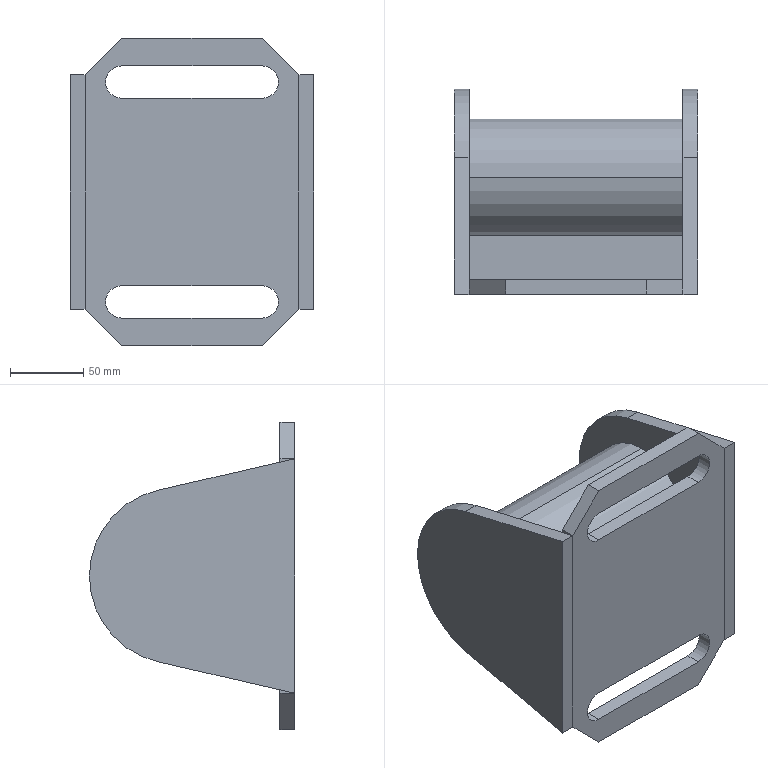Part | SolidWorks | features MirrorStock 1 | 5 solids | 42 faces | box 166 x 140 x 210 mm | volume 892301 mm3 | plane 31 | cylinder 11 | commonest cylinder face diameters 22 x4 80 x3 64 x2 120 x2
STEP:
#1=CARTESIAN_POINT('',(-48.,10.,105.));
#2=VERTEX_POINT('',#1);
#3=CARTESIAN_POINT('',(-73.,10.,80.));
#4=VERTEX_POINT('',#3);
#5=CARTESIAN_POINT('',(-73.,10.,80.));
#6=DIRECTION('',(-0.7071,0.,-0.7071));
#7=VECTOR('',#6,1000.);
#8=LINE('',#5,#7);
#9=EDGE_CURVE('',#2,#4,#8,.T.);
#10=ORIENTED_EDGE('',*,*,#9,.F.);
#11=CARTESIAN_POINT('',(48.,10.,105.));
#12=VERTEX_POINT('',#11);
#13=CARTESIAN_POINT('',(-48.,10.,105.));
#14=DIRECTION('',(-1.,0.,0.));
#15=VECTOR('',#14,1000.);
#16=LINE('',#13,#15);
#17=EDGE_CURVE('',#12,#2,#16,.T.);
#18=ORIENTED_EDGE('',*,*,#17,.F.);
#19=CARTESIAN_POINT('',(73.,10.,80.));
#20=VERTEX_POINT('',#19);
#21=CARTESIAN_POINT('',(73.,10.,80.));
#22=DIRECTION('',(-0.7071,0.,0.7071));
#23=VECTOR('',#22,1000.);
#24=LINE('',#21,#23);
#25=EDGE_CURVE('',#20,#12,#24,.T.);
#26=ORIENTED_EDGE('',*,*,#25,.F.);
#27=CARTESIAN_POINT('',(73.,10.,-80.));
#28=VERTEX_POINT('',#27);
#29=CARTESIAN_POINT('',(73.,10.,-80.));
#30=DIRECTION('',(0.,0.,1.));
#31=VECTOR('',#30,1000.);
#32=LINE('',#29,#31);
#33=EDGE_CURVE('',#28,#20,#32,.T.);
#34=ORIENTED_EDGE('',*,*,#33,.F.);
#35=CARTESIAN_POINT('',(48.,10.,-105.));
#36=VERTEX_POINT('',#35);
#37=CARTESIAN_POINT('',(73.,10.,-80.));
#38=DIRECTION('',(0.7071,0.,0.7071));
#39=VECTOR('',#38,1000.);
#40=LINE('',#37,#39);
#41=EDGE_CURVE('',#36,#28,#40,.T.);
#42=ORIENTED_EDGE('',*,*,#41,.F.);
#43=CARTESIAN_POINT('',(-48.,10.,-105.));
#44=VERTEX_POINT('',#43);
#45=CARTESIAN_POINT('',(-48.,10.,-105.));
#46=DIRECTION('',(1.,0.,0.));
#47=VECTOR('',#46,1000.);
#48=LINE('',#45,#47);
#49=EDGE_CURVE('',#44,#36,#48,.T.);
#50=ORIENTED_EDGE('',*,*,#49,.F.);
#51=CARTESIAN_POINT('',(-73.,10.,-80.));
#52=VERTEX_POINT('',#51);
#53=CARTESIAN_POINT('',(-73.,10.,-80.));
#54=DIRECTION('',(0.7071,0.,-0.7071));
#55=VECTOR('',#54,1000.);
#56=LINE('',#53,#55);
#57=EDGE_CURVE('',#52,#44,#56,.T.);
#58=ORIENTED_EDGE('',*,*,#57,.F.);
#59=CARTESIAN_POINT('',(-73.,10.,-80.));
#60=DIRECTION('',(0.,0.,-1.));
#61=VECTOR('',#60,1000.);
#62=LINE('',#59,#61);
#63=EDGE_CURVE('',#4,#52,#62,.T.);
#64=ORIENTED_EDGE('',*,*,#63,.F.);
#65=EDGE_LOOP('',(#10,#18,#26,#34,#42,#50,#58,#64));
#66=FACE_OUTER_BOUND('',#65,.T.);
#67=CARTESIAN_POINT('',(-48.,10.,64.));
#68=VERTEX_POINT('',#67);
#69=CARTESIAN_POINT('',(48.,10.,64.));
#70=VERTEX_POINT('',#69);
#71=CARTESIAN_POINT('',(-48.,10.,64.));
#72=DIRECTION('',(1.,0.,0.));
#73=VECTOR('',#72,1000.);
#74=LINE('',#71,#73);
#75=EDGE_CURVE('',#68,#70,#74,.T.);
#76=ORIENTED_EDGE('',*,*,#75,.T.);
#77=CARTESIAN_POINT('',(48.,10.,86.));
#78=VERTEX_POINT('',#77);
#79=CARTESIAN_POINT('',(48.,10.,75.));
#80=DIRECTION('',(0.,-1.,0.));
#81=DIRECTION('',(0.,0.,-1.));
#82=AXIS2_PLACEMENT_3D('',#79,#80,#81);
#83=CIRCLE('',#82,11.);
#84=EDGE_CURVE('',#70,#78,#83,.T.);
#85=ORIENTED_EDGE('',*,*,#84,.T.);
#86=CARTESIAN_POINT('',(-48.,10.,86.));
#87=VERTEX_POINT('',#86);
#88=CARTESIAN_POINT('',(-48.,10.,86.));
#89=DIRECTION('',(-1.,0.,0.));
#90=VECTOR('',#89,1000.);
#91=LINE('',#88,#90);
#92=EDGE_CURVE('',#78,#87,#91,.T.);
#93=ORIENTED_EDGE('',*,*,#92,.T.);
#94=CARTESIAN_POINT('',(-48.,10.,75.));
#95=DIRECTION('',(0.,-1.,0.));
#96=DIRECTION('',(0.,0.,-1.));
#97=AXIS2_PLACEMENT_3D('',#94,#95,#96);
#98=CIRCLE('',#97,11.);
#99=EDGE_CURVE('',#87,#68,#98,.T.);
#100=ORIENTED_EDGE('',*,*,#99,.T.);
#101=EDGE_LOOP('',(#76,#85,#93,#100));
#102=FACE_BOUND('',#101,.T.);
#103=CARTESIAN_POINT('',(-48.,10.,-86.));
#104=VERTEX_POINT('',#103);
#105=CARTESIAN_POINT('',(48.,10.,-86.));
#106=VERTEX_POINT('',#105);
#107=CARTESIAN_POINT('',(-48.,10.,-86.));
#108=DIRECTION('',(1.,0.,0.));
#109=VECTOR('',#108,1000.);
#110=LINE('',#107,#109);
#111=EDGE_CURVE('',#104,#106,#110,.T.);
#112=ORIENTED_EDGE('',*,*,#111,.T.);
#113=CARTESIAN_POINT('',(48.,10.,-64.));
#114=VERTEX_POINT('',#113);
#115=CARTESIAN_POINT('',(48.,10.,-75.));
#116=DIRECTION('',(0.,-1.,0.));
#117=DIRECTION('',(0.,0.,1.));
#118=AXIS2_PLACEMENT_3D('',#115,#116,#117);
#119=CIRCLE('',#118,11.);
#120=EDGE_CURVE('',#106,#114,#119,.T.);
#121=ORIENTED_EDGE('',*,*,#120,.T.);
#122=CARTESIAN_POINT('',(-48.,10.,-64.));
#123=VERTEX_POINT('',#122);
#124=CARTESIAN_POINT('',(-48.,10.,-64.));
#125=DIRECTION('',(-1.,0.,0.));
#126=VECTOR('',#125,1000.);
#127=LINE('',#124,#126);
#128=EDGE_CURVE('',#114,#123,#127,.T.);
#129=ORIENTED_EDGE('',*,*,#128,.T.);
#130=CARTESIAN_POINT('',(-48.,10.,-75.));
#131=DIRECTION('',(0.,-1.,0.));
#132=DIRECTION('',(0.,0.,1.));
#133=AXIS2_PLACEMENT_3D('',#130,#131,#132);
#134=CIRCLE('',#133,11.);
#135=EDGE_CURVE('',#123,#104,#134,.T.);
#136=ORIENTED_EDGE('',*,*,#135,.T.);
#137=EDGE_LOOP('',(#112,#121,#129,#136));
#138=FACE_BOUND('',#137,.T.);
#139=CARTESIAN_POINT('',(0.,10.,0.));
#140=DIRECTION('',(0.,1.,0.));
#141=DIRECTION('',(0.,0.,-1.));
#142=AXIS2_PLACEMENT_3D('',#139,#140,#141);
#143=PLANE('',#142);
#144=ADVANCED_FACE('',(#66,#102,#138),#143,.T.);
#145=CARTESIAN_POINT('',(-48.,0.,86.));
#146=VERTEX_POINT('',#145);
#147=CARTESIAN_POINT('',(-48.,0.,64.));
#148=VERTEX_POINT('',#147);
#149=CARTESIAN_POINT('',(-48.,0.,75.));
#150=DIRECTION('',(0.,-1.,0.));
#151=DIRECTION('',(0.,0.,-1.));
#152=AXIS2_PLACEMENT_3D('',#149,#150,#151);
#153=CIRCLE('',#152,11.);
#154=EDGE_CURVE('',#146,#148,#153,.T.);
#155=ORIENTED_EDGE('',*,*,#154,.F.);
#156=CARTESIAN_POINT('',(48.,0.,86.));
#157=VERTEX_POINT('',#156);
#158=CARTESIAN_POINT('',(-48.,0.,86.));
#159=DIRECTION('',(-1.,0.,0.));
#160=VECTOR('',#159,1000.);
#161=LINE('',#158,#160);
#162=EDGE_CURVE('',#157,#146,#161,.T.);
#163=ORIENTED_EDGE('',*,*,#162,.F.);
#164=CARTESIAN_POINT('',(48.,0.,64.));
#165=VERTEX_POINT('',#164);
#166=CARTESIAN_POINT('',(48.,0.,75.));
#167=DIRECTION('',(0.,-1.,0.));
#168=DIRECTION('',(0.,0.,-1.));
#169=AXIS2_PLACEMENT_3D('',#166,#167,#168);
#170=CIRCLE('',#169,11.);
#171=EDGE_CURVE('',#165,#157,#170,.T.);
#172=ORIENTED_EDGE('',*,*,#171,.F.);
#173=CARTESIAN_POINT('',(-48.,0.,64.));
#174=DIRECTION('',(1.,0.,0.));
#175=VECTOR('',#174,1000.);
#176=LINE('',#173,#175);
#177=EDGE_CURVE('',#148,#165,#176,.T.);
#178=ORIENTED_EDGE('',*,*,#177,.F.);
#179=EDGE_LOOP('',(#155,#163,#172,#178));
#180=FACE_BOUND('',#179,.T.);
#181=CARTESIAN_POINT('',(-48.,0.,105.));
#182=VERTEX_POINT('',#181);
#183=CARTESIAN_POINT('',(-73.,0.,80.));
#184=VERTEX_POINT('',#183);
#185=CARTESIAN_POINT('',(-73.,0.,80.));
#186=DIRECTION('',(-0.7071,0.,-0.7071));
#187=VECTOR('',#186,1000.);
#188=LINE('',#185,#187);
#189=EDGE_CURVE('',#182,#184,#188,.T.);
#190=ORIENTED_EDGE('',*,*,#189,.T.);
#191=CARTESIAN_POINT('',(-73.,0.,-80.));
#192=VERTEX_POINT('',#191);
#193=CARTESIAN_POINT('',(-73.,0.,-80.));
#194=DIRECTION('',(0.,0.,-1.));
#195=VECTOR('',#194,1000.);
#196=LINE('',#193,#195);
#197=EDGE_CURVE('',#184,#192,#196,.T.);
#198=ORIENTED_EDGE('',*,*,#197,.T.);
#199=CARTESIAN_POINT('',(-48.,0.,-105.));
#200=VERTEX_POINT('',#199);
#201=CARTESIAN_POINT('',(-73.,0.,-80.));
#202=DIRECTION('',(0.7071,0.,-0.7071));
#203=VECTOR('',#202,1000.);
#204=LINE('',#201,#203);
#205=EDGE_CURVE('',#192,#200,#204,.T.);
#206=ORIENTED_EDGE('',*,*,#205,.T.);
#207=CARTESIAN_POINT('',(48.,0.,-105.));
#208=VERTEX_POINT('',#207);
#209=CARTESIAN_POINT('',(-48.,0.,-105.));
#210=DIRECTION('',(1.,0.,0.));
#211=VECTOR('',#210,1000.);
#212=LINE('',#209,#211);
#213=EDGE_CURVE('',#200,#208,#212,.T.);
#214=ORIENTED_EDGE('',*,*,#213,.T.);
#215=CARTESIAN_POINT('',(73.,0.,-80.));
#216=VERTEX_POINT('',#215);
#217=CARTESIAN_POINT('',(73.,0.,-80.));
#218=DIRECTION('',(0.7071,0.,0.7071));
#219=VECTOR('',#218,1000.);
#220=LINE('',#217,#219);
#221=EDGE_CURVE('',#208,#216,#220,.T.);
#222=ORIENTED_EDGE('',*,*,#221,.T.);
#223=CARTESIAN_POINT('',(73.,0.,80.));
#224=VERTEX_POINT('',#223);
#225=CARTESIAN_POINT('',(73.,0.,-80.));
#226=DIRECTION('',(0.,0.,1.));
#227=VECTOR('',#226,1000.);
#228=LINE('',#225,#227);
#229=EDGE_CURVE('',#216,#224,#228,.T.);
#230=ORIENTED_EDGE('',*,*,#229,.T.);
#231=CARTESIAN_POINT('',(48.,0.,105.));
#232=VERTEX_POINT('',#231);
#233=CARTESIAN_POINT('',(73.,0.,80.));
#234=DIRECTION('',(-0.7071,0.,0.7071));
#235=VECTOR('',#234,1000.);
#236=LINE('',#233,#235);
#237=EDGE_CURVE('',#224,#232,#236,.T.);
#238=ORIENTED_EDGE('',*,*,#237,.T.);
#239=CARTESIAN_POINT('',(-48.,0.,105.));
#240=DIRECTION('',(-1.,0.,0.));
#241=VECTOR('',#240,1000.);
#242=LINE('',#239,#241);
#243=EDGE_CURVE('',#232,#182,#242,.T.);
#244=ORIENTED_EDGE('',*,*,#243,.T.);
#245=EDGE_LOOP('',(#190,#198,#206,#214,#222,#230,#238,#244));
#246=FACE_OUTER_BOUND('',#245,.T.);
#247=CARTESIAN_POINT('',(-48.,0.,-64.));
#248=VERTEX_POINT('',#247);
#249=CARTESIAN_POINT('',(-48.,0.,-86.));
#250=VERTEX_POINT('',#249);
#251=CARTESIAN_POINT('',(-48.,0.,-75.));
#252=DIRECTION('',(0.,-1.,0.));
#253=DIRECTION('',(0.,0.,1.));
#254=AXIS2_PLACEMENT_3D('',#251,#252,#253);
#255=CIRCLE('',#254,11.);
#256=EDGE_CURVE('',#248,#250,#255,.T.);
#257=ORIENTED_EDGE('',*,*,#256,.F.);
#258=CARTESIAN_POINT('',(48.,0.,-64.));
#259=VERTEX_POINT('',#258);
#260=CARTESIAN_POINT('',(-48.,0.,-64.));
#261=DIRECTION('',(-1.,0.,0.));
#262=VECTOR('',#261,1000.);
#263=LINE('',#260,#262);
#264=EDGE_CURVE('',#259,#248,#263,.T.);
#265=ORIENTED_EDGE('',*,*,#264,.F.);
#266=CARTESIAN_POINT('',(48.,0.,-86.));
#267=VERTEX_POINT('',#266);
#268=CARTESIAN_POINT('',(48.,0.,-75.));
#269=DIRECTION('',(0.,-1.,0.));
#270=DIRECTION('',(0.,0.,1.));
#271=AXIS2_PLACEMENT_3D('',#268,#269,#270);
#272=CIRCLE('',#271,11.);
#273=EDGE_CURVE('',#267,#259,#272,.T.);
#274=ORIENTED_EDGE('',*,*,#273,.F.);
#275=CARTESIAN_POINT('',(-48.,0.,-86.));
#276=DIRECTION('',(1.,0.,0.));
#277=VECTOR('',#276,1000.);
#278=LINE('',#275,#277);
#279=EDGE_CURVE('',#250,#267,#278,.T.);
#280=ORIENTED_EDGE('',*,*,#279,.F.);
#281=EDGE_LOOP('',(#257,#265,#274,#280));
#282=FACE_BOUND('',#281,.T.);
#283=CARTESIAN_POINT('',(0.,0.,0.));
#284=DIRECTION('',(0.,1.,0.));
#285=DIRECTION('',(0.,0.,-1.));
#286=AXIS2_PLACEMENT_3D('',#283,#284,#285);
#287=PLANE('',#286);
#288=ADVANCED_FACE('',(#180,#246,#282),#287,.F.);
#289=ORIENTED_EDGE('',*,*,#189,.F.);
#290=CARTESIAN_POINT('',(-48.,10.,105.));
#291=DIRECTION('',(0.,-1.,0.));
#292=VECTOR('',#291,1000.);
#293=LINE('',#290,#292);
#294=EDGE_CURVE('',#2,#182,#293,.T.);
#295=ORIENTED_EDGE('',*,*,#294,.F.);
#296=ORIENTED_EDGE('',*,*,#9,.T.);
#297=CARTESIAN_POINT('',(-73.,10.,80.));
#298=DIRECTION('',(0.,-1.,0.));
#299=VECTOR('',#298,1000.);
#300=LINE('',#297,#299);
#301=EDGE_CURVE('',#4,#184,#300,.T.);
#302=ORIENTED_EDGE('',*,*,#301,.T.);
#303=EDGE_LOOP('',(#289,#295,#296,#302));
#304=FACE_OUTER_BOUND('',#303,.T.);
#305=CARTESIAN_POINT('',(-73.,10.,80.));
#306=DIRECTION('',(0.7071,0.,-0.7071));
#307=DIRECTION('',(0.7071,0.,0.7071));
#308=AXIS2_PLACEMENT_3D('',#305,#306,#307);
#309=PLANE('',#308);
#310=ADVANCED_FACE('',(#304),#309,.F.);
#311=ORIENTED_EDGE('',*,*,#197,.F.);
#312=ORIENTED_EDGE('',*,*,#301,.F.);
#313=ORIENTED_EDGE('',*,*,#63,.T.);
#314=CARTESIAN_POINT('',(-73.,10.,-80.));
#315=DIRECTION('',(0.,-1.,0.));
#316=VECTOR('',#315,1000.);
#317=LINE('',#314,#316);
#318=EDGE_CURVE('',#52,#192,#317,.T.);
#319=ORIENTED_EDGE('',*,*,#318,.T.);
#320=EDGE_LOOP('',(#311,#312,#313,#319));
#321=FACE_OUTER_BOUND('',#320,.T.);
#322=CARTESIAN_POINT('',(-73.,10.,-80.));
#323=DIRECTION('',(1.,0.,0.));
#324=DIRECTION('',(0.,0.,1.));
#325=AXIS2_PLACEMENT_3D('',#322,#323,#324);
#326=PLANE('',#325);
#327=ADVANCED_FACE('',(#321),#326,.F.);
#328=ORIENTED_EDGE('',*,*,#205,.F.);
#329=ORIENTED_EDGE('',*,*,#318,.F.);
#330=ORIENTED_EDGE('',*,*,#57,.T.);
#331=CARTESIAN_POINT('',(-48.,10.,-105.));
#332=DIRECTION('',(0.,-1.,0.));
#333=VECTOR('',#332,1000.);
#334=LINE('',#331,#333);
#335=EDGE_CURVE('',#44,#200,#334,.T.);
#336=ORIENTED_EDGE('',*,*,#335,.T.);
#337=EDGE_LOOP('',(#328,#329,#330,#336));
#338=FACE_OUTER_BOUND('',#337,.T.);
#339=CARTESIAN_POINT('',(-73.,10.,-80.));
#340=DIRECTION('',(0.7071,0.,0.7071));
#341=DIRECTION('',(-0.7071,0.,0.7071));
#342=AXIS2_PLACEMENT_3D('',#339,#340,#341);
#343=PLANE('',#342);
#344=ADVANCED_FACE('',(#338),#343,.F.);
#345=ORIENTED_EDGE('',*,*,#213,.F.);
#346=ORIENTED_EDGE('',*,*,#335,.F.);
#347=ORIENTED_EDGE('',*,*,#49,.T.);
#348=CARTESIAN_POINT('',(48.,10.,-105.));
#349=DIRECTION('',(0.,-1.,0.));
#350=VECTOR('',#349,1000.);
#351=LINE('',#348,#350);
#352=EDGE_CURVE('',#36,#208,#351,.T.);
#353=ORIENTED_EDGE('',*,*,#352,.T.);
#354=EDGE_LOOP('',(#345,#346,#347,#353));
#355=FACE_OUTER_BOUND('',#354,.T.);
#356=CARTESIAN_POINT('',(-48.,10.,-105.));
#357=DIRECTION('',(0.,0.,1.));
#358=DIRECTION('',(-1.,0.,0.));
#359=AXIS2_PLACEMENT_3D('',#356,#357,#358);
#360=PLANE('',#359);
#361=ADVANCED_FACE('',(#355),#360,.F.);
#362=ORIENTED_EDGE('',*,*,#221,.F.);
#363=ORIENTED_EDGE('',*,*,#352,.F.);
#364=ORIENTED_EDGE('',*,*,#41,.T.);
#365=CARTESIAN_POINT('',(73.,10.,-80.));
#366=DIRECTION('',(0.,-1.,0.));
#367=VECTOR('',#366,1000.);
#368=LINE('',#365,#367);
#369=EDGE_CURVE('',#28,#216,#368,.T.);
#370=ORIENTED_EDGE('',*,*,#369,.T.);
#371=EDGE_LOOP('',(#362,#363,#364,#370));
#372=FACE_OUTER_BOUND('',#371,.T.);
#373=CARTESIAN_POINT('',(73.,10.,-80.));
#374=DIRECTION('',(-0.7071,0.,0.7071));
#375=DIRECTION('',(-0.7071,0.,-0.7071));
#376=AXIS2_PLACEMENT_3D('',#373,#374,#375);
#377=PLANE('',#376);
#378=ADVANCED_FACE('',(#372),#377,.F.);
#379=ORIENTED_EDGE('',*,*,#229,.F.);
#380=ORIENTED_EDGE('',*,*,#369,.F.);
#381=ORIENTED_EDGE('',*,*,#33,.T.);
#382=CARTESIAN_POINT('',(73.,10.,80.));
#383=DIRECTION('',(0.,-1.,0.));
#384=VECTOR('',#383,1000.);
#385=LINE('',#382,#384);
#386=EDGE_CURVE('',#20,#224,#385,.T.);
#387=ORIENTED_EDGE('',*,*,#386,.T.);
#388=EDGE_LOOP('',(#379,#380,#381,#387));
#389=FACE_OUTER_BOUND('',#388,.T.);
#390=CARTESIAN_POINT('',(73.,10.,-80.));
#391=DIRECTION('',(-1.,0.,0.));
#392=DIRECTION('',(0.,0.,-1.));
#393=AXIS2_PLACEMENT_3D('',#390,#391,#392);
#394=PLANE('',#393);
#395=ADVANCED_FACE('',(#389),#394,.F.);
#396=ORIENTED_EDGE('',*,*,#237,.F.);
#397=ORIENTED_EDGE('',*,*,#386,.F.);
#398=ORIENTED_EDGE('',*,*,#25,.T.);
#399=CARTESIAN_POINT('',(48.,10.,105.));
#400=DIRECTION('',(0.,-1.,0.));
#401=VECTOR('',#400,1000.);
#402=LINE('',#399,#401);
#403=EDGE_CURVE('',#12,#232,#402,.T.);
#404=ORIENTED_EDGE('',*,*,#403,.T.);
#405=EDGE_LOOP('',(#396,#397,#398,#404));
#406=FACE_OUTER_BOUND('',#405,.T.);
#407=CARTESIAN_POINT('',(73.,10.,80.));
#408=DIRECTION('',(-0.7071,0.,-0.7071));
#409=DIRECTION('',(0.7071,0.,-0.7071));
#410=AXIS2_PLACEMENT_3D('',#407,#408,#409);
#411=PLANE('',#410);
#412=ADVANCED_FACE('',(#406),#411,.F.);
#413=ORIENTED_EDGE('',*,*,#243,.F.);
#414=ORIENTED_EDGE('',*,*,#403,.F.);
#415=ORIENTED_EDGE('',*,*,#17,.T.);
#416=ORIENTED_EDGE('',*,*,#294,.T.);
#417=EDGE_LOOP('',(#413,#414,#415,#416));
#418=FACE_OUTER_BOUND('',#417,.T.);
#419=CARTESIAN_POINT('',(-48.,10.,105.));
#420=DIRECTION('',(0.,0.,-1.));
#421=DIRECTION('',(1.,0.,0.));
#422=AXIS2_PLACEMENT_3D('',#419,#420,#421);
#423=PLANE('',#422);
#424=ADVANCED_FACE('',(#418),#423,.F.);
#425=ORIENTED_EDGE('',*,*,#154,.T.);
#426=CARTESIAN_POINT('',(-48.,10.,64.));
#427=DIRECTION('',(0.,-1.,0.));
#428=VECTOR('',#427,1000.);
#429=LINE('',#426,#428);
#430=EDGE_CURVE('',#68,#148,#429,.T.);
#431=ORIENTED_EDGE('',*,*,#430,.F.);
#432=ORIENTED_EDGE('',*,*,#99,.F.);
#433=CARTESIAN_POINT('',(-48.,10.,86.));
#434=DIRECTION('',(0.,-1.,0.));
#435=VECTOR('',#434,1000.);
#436=LINE('',#433,#435);
#437=EDGE_CURVE('',#87,#146,#436,.T.);
#438=ORIENTED_EDGE('',*,*,#437,.T.);
#439=EDGE_LOOP('',(#425,#431,#432,#438));
#440=FACE_OUTER_BOUND('',#439,.T.);
#441=CARTESIAN_POINT('',(-48.,10.,75.));
#442=DIRECTION('',(0.,-1.,0.));
#443=DIRECTION('',(0.,0.,1.));
#444=AXIS2_PLACEMENT_3D('',#441,#442,#443);
#445=CYLINDRICAL_SURFACE('',#444,11.);
#446=ADVANCED_FACE('',(#440),#445,.F.);
#447=ORIENTED_EDGE('',*,*,#177,.T.);
#448=CARTESIAN_POINT('',(48.,10.,64.));
#449=DIRECTION('',(0.,-1.,0.));
#450=VECTOR('',#449,1000.);
#451=LINE('',#448,#450);
#452=EDGE_CURVE('',#70,#165,#451,.T.);
#453=ORIENTED_EDGE('',*,*,#452,.F.);
#454=ORIENTED_EDGE('',*,*,#75,.F.);
#455=ORIENTED_EDGE('',*,*,#430,.T.);
#456=EDGE_LOOP('',(#447,#453,#454,#455));
#457=FACE_OUTER_BOUND('',#456,.T.);
#458=CARTESIAN_POINT('',(-48.,10.,64.));
#459=DIRECTION('',(0.,0.,1.));
#460=DIRECTION('',(-1.,0.,0.));
#461=AXIS2_PLACEMENT_3D('',#458,#459,#460);
#462=PLANE('',#461);
#463=ADVANCED_FACE('',(#457),#462,.T.);
#464=ORIENTED_EDGE('',*,*,#171,.T.);
#465=CARTESIAN_POINT('',(48.,10.,86.));
#466=DIRECTION('',(0.,-1.,0.));
#467=VECTOR('',#466,1000.);
#468=LINE('',#465,#467);
#469=EDGE_CURVE('',#78,#157,#468,.T.);
#470=ORIENTED_EDGE('',*,*,#469,.F.);
#471=ORIENTED_EDGE('',*,*,#84,.F.);
#472=ORIENTED_EDGE('',*,*,#452,.T.);
#473=EDGE_LOOP('',(#464,#470,#471,#472));
#474=FACE_OUTER_BOUND('',#473,.T.);
#475=CARTESIAN_POINT('',(48.,10.,75.));
#476=DIRECTION('',(0.,-1.,0.));
#477=DIRECTION('',(0.,0.,1.));
#478=AXIS2_PLACEMENT_3D('',#475,#476,#477);
#479=CYLINDRICAL_SURFACE('',#478,11.);
#480=ADVANCED_FACE('',(#474),#479,.F.);
#481=ORIENTED_EDGE('',*,*,#162,.T.);
#482=ORIENTED_EDGE('',*,*,#437,.F.);
#483=ORIENTED_EDGE('',*,*,#92,.F.);
#484=ORIENTED_EDGE('',*,*,#469,.T.);
#485=EDGE_LOOP('',(#481,#482,#483,#484));
#486=FACE_OUTER_BOUND('',#485,.T.);
#487=CARTESIAN_POINT('',(-48.,10.,86.));
#488=DIRECTION('',(0.,0.,-1.));
#489=DIRECTION('',(1.,0.,0.));
#490=AXIS2_PLACEMENT_3D('',#487,#488,#489);
#491=PLANE('',#490);
#492=ADVANCED_FACE('',(#486),#491,.T.);
#493=ORIENTED_EDGE('',*,*,#256,.T.);
#494=CARTESIAN_POINT('',(-48.,10.,-86.));
#495=DIRECTION('',(0.,-1.,0.));
#496=VECTOR('',#495,1000.);
#497=LINE('',#494,#496);
#498=EDGE_CURVE('',#104,#250,#497,.T.);
#499=ORIENTED_EDGE('',*,*,#498,.F.);
#500=ORIENTED_EDGE('',*,*,#135,.F.);
#501=CARTESIAN_POINT('',(-48.,10.,-64.));
#502=DIRECTION('',(0.,-1.,0.));
#503=VECTOR('',#502,1000.);
#504=LINE('',#501,#503);
#505=EDGE_CURVE('',#123,#248,#504,.T.);
#506=ORIENTED_EDGE('',*,*,#505,.T.);
#507=EDGE_LOOP('',(#493,#499,#500,#506));
#508=FACE_OUTER_BOUND('',#507,.T.);
#509=CARTESIAN_POINT('',(-48.,10.,-75.));
#510=DIRECTION('',(0.,-1.,0.));
#511=DIRECTION('',(0.,0.,1.));
#512=AXIS2_PLACEMENT_3D('',#509,#510,#511);
#513=CYLINDRICAL_SURFACE('',#512,11.);
#514=ADVANCED_FACE('',(#508),#513,.F.);
#515=ORIENTED_EDGE('',*,*,#279,.T.);
#516=CARTESIAN_POINT('',(48.,10.,-86.));
#517=DIRECTION('',(0.,-1.,0.));
#518=VECTOR('',#517,1000.);
#519=LINE('',#516,#518);
#520=EDGE_CURVE('',#106,#267,#519,.T.);
#521=ORIENTED_EDGE('',*,*,#520,.F.);
#522=ORIENTED_EDGE('',*,*,#111,.F.);
#523=ORIENTED_EDGE('',*,*,#498,.T.);
#524=EDGE_LOOP('',(#515,#521,#522,#523));
#525=FACE_OUTER_BOUND('',#524,.T.);
#526=CARTESIAN_POINT('',(-48.,10.,-86.));
#527=DIRECTION('',(0.,0.,1.));
#528=DIRECTION('',(-1.,0.,0.));
#529=AXIS2_PLACEMENT_3D('',#526,#527,#528);
#530=PLANE('',#529);
#531=ADVANCED_FACE('',(#525),#530,.T.);
#532=ORIENTED_EDGE('',*,*,#273,.T.);
#533=CARTESIAN_POINT('',(48.,10.,-64.));
#534=DIRECTION('',(0.,-1.,0.));
#535=VECTOR('',#534,1000.);
#536=LINE('',#533,#535);
#537=EDGE_CURVE('',#114,#259,#536,.T.);
#538=ORIENTED_EDGE('',*,*,#537,.F.);
#539=ORIENTED_EDGE('',*,*,#120,.F.);
#540=ORIENTED_EDGE('',*,*,#520,.T.);
#541=EDGE_LOOP('',(#532,#538,#539,#540));
#542=FACE_OUTER_BOUND('',#541,.T.);
#543=CARTESIAN_POINT('',(48.,10.,-75.));
#544=DIRECTION('',(0.,-1.,0.));
#545=DIRECTION('',(0.,0.,1.));
#546=AXIS2_PLACEMENT_3D('',#543,#544,#545);
#547=CYLINDRICAL_SURFACE('',#546,11.);
#548=ADVANCED_FACE('',(#542),#547,.F.);
#549=ORIENTED_EDGE('',*,*,#264,.T.);
#550=ORIENTED_EDGE('',*,*,#505,.F.);
#551=ORIENTED_EDGE('',*,*,#128,.F.);
#552=ORIENTED_EDGE('',*,*,#537,.T.);
#553=EDGE_LOOP('',(#549,#550,#551,#552));
#554=FACE_OUTER_BOUND('',#553,.T.);
#555=CARTESIAN_POINT('',(-48.,10.,-64.));
#556=DIRECTION('',(0.,0.,-1.));
#557=DIRECTION('',(1.,0.,0.));
#558=AXIS2_PLACEMENT_3D('',#555,#556,#557);
#559=PLANE('',#558);
#560=ADVANCED_FACE('',(#554),#559,.T.);
#561=CLOSED_SHELL('',(#144,#288,#310,#327,#344,#361,#378,#395,#412,#424,#446,#463,#480,#492,#514,#531,#548,#560));
#562=MANIFOLD_SOLID_BREP('',#561);
#563=CARTESIAN_POINT('',(-73.,0.,80.));
#564=VERTEX_POINT('',#563);
#565=CARTESIAN_POINT('',(-73.,0.,-80.));
#566=VERTEX_POINT('',#565);
#567=CARTESIAN_POINT('',(-73.,0.,80.));
#568=DIRECTION('',(0.,0.,-1.));
#569=VECTOR('',#568,1000.);
#570=LINE('',#567,#569);
#571=EDGE_CURVE('',#564,#566,#570,.T.);
#572=ORIENTED_EDGE('',*,*,#571,.F.);
#573=CARTESIAN_POINT('',(-83.,0.,80.));
#574=VERTEX_POINT('',#573);
#575=CARTESIAN_POINT('',(-83.,0.,80.));
#576=DIRECTION('',(1.,0.,0.));
#577=VECTOR('',#576,1000.);
#578=LINE('',#575,#577);
#579=EDGE_CURVE('',#574,#564,#578,.T.);
#580=ORIENTED_EDGE('',*,*,#579,.F.);
#581=CARTESIAN_POINT('',(-83.,0.,-80.));
#582=VERTEX_POINT('',#581);
#583=CARTESIAN_POINT('',(-83.,0.,80.));
#584=DIRECTION('',(0.,0.,-1.));
#585=VECTOR('',#584,1000.);
#586=LINE('',#583,#585);
#587=EDGE_CURVE('',#574,#582,#586,.T.);
#588=ORIENTED_EDGE('',*,*,#587,.T.);
#589=CARTESIAN_POINT('',(-83.,0.,-80.));
#590=DIRECTION('',(1.,0.,0.));
#591=VECTOR('',#590,1000.);
#592=LINE('',#589,#591);
#593=EDGE_CURVE('',#582,#566,#592,.T.);
#594=ORIENTED_EDGE('',*,*,#593,.T.);
#595=EDGE_LOOP('',(#572,#580,#588,#594));
#596=FACE_OUTER_BOUND('',#595,.T.);
#597=CARTESIAN_POINT('',(-83.,0.,80.));
#598=DIRECTION('',(0.,1.,0.));
#599=DIRECTION('',(0.,0.,-1.));
#600=AXIS2_PLACEMENT_3D('',#597,#598,#599);
#601=PLANE('',#600);
#602=ADVANCED_FACE('',(#596),#601,.F.);
#603=CARTESIAN_POINT('',(-73.,93.469,-58.469));
#604=VERTEX_POINT('',#603);
#605=CARTESIAN_POINT('',(-73.,0.,-80.));
#606=DIRECTION('',(0.,0.9745,0.2245));
#607=VECTOR('',#606,1000.);
#608=LINE('',#605,#607);
#609=EDGE_CURVE('',#566,#604,#608,.T.);
#610=ORIENTED_EDGE('',*,*,#609,.F.);
#611=ORIENTED_EDGE('',*,*,#593,.F.);
#612=CARTESIAN_POINT('',(-83.,93.469,-58.469));
#613=VERTEX_POINT('',#612);
#614=CARTESIAN_POINT('',(-83.,0.,-80.));
#615=DIRECTION('',(0.,0.9745,0.2245));
#616=VECTOR('',#615,1000.);
#617=LINE('',#614,#616);
#618=EDGE_CURVE('',#582,#613,#617,.T.);
#619=ORIENTED_EDGE('',*,*,#618,.T.);
#620=CARTESIAN_POINT('',(-83.,93.469,-58.469));
#621=DIRECTION('',(1.,0.,0.));
#622=VECTOR('',#621,1000.);
#623=LINE('',#620,#622);
#624=EDGE_CURVE('',#613,#604,#623,.T.);
#625=ORIENTED_EDGE('',*,*,#624,.T.);
#626=EDGE_LOOP('',(#610,#611,#619,#625));
#627=FACE_OUTER_BOUND('',#626,.T.);
#628=CARTESIAN_POINT('',(-83.,0.,-80.));
#629=DIRECTION('',(0.,-0.2245,0.9745));
#630=DIRECTION('',(0.,0.9745,0.2245));
#631=AXIS2_PLACEMENT_3D('',#628,#629,#630);
#632=PLANE('',#631);
#633=ADVANCED_FACE('',(#627),#632,.F.);
#634=CARTESIAN_POINT('',(-73.,93.469,58.469));
#635=VERTEX_POINT('',#634);
#636=CARTESIAN_POINT('',(-73.,80.,0.));
#637=DIRECTION('',(1.,0.,0.));
#638=DIRECTION('',(0.,0.,-1.));
#639=AXIS2_PLACEMENT_3D('',#636,#637,#638);
#640=CIRCLE('',#639,60.);
#641=EDGE_CURVE('',#604,#635,#640,.T.);
#642=ORIENTED_EDGE('',*,*,#641,.F.);
#643=ORIENTED_EDGE('',*,*,#624,.F.);
#644=CARTESIAN_POINT('',(-83.,93.469,58.469));
#645=VERTEX_POINT('',#644);
#646=CARTESIAN_POINT('',(-83.,80.,0.));
#647=DIRECTION('',(1.,0.,0.));
#648=DIRECTION('',(0.,0.,-1.));
#649=AXIS2_PLACEMENT_3D('',#646,#647,#648);
#650=CIRCLE('',#649,60.);
#651=EDGE_CURVE('',#613,#645,#650,.T.);
#652=ORIENTED_EDGE('',*,*,#651,.T.);
#653=CARTESIAN_POINT('',(-83.,93.469,58.469));
#654=DIRECTION('',(1.,0.,0.));
#655=VECTOR('',#654,1000.);
#656=LINE('',#653,#655);
#657=EDGE_CURVE('',#645,#635,#656,.T.);
#658=ORIENTED_EDGE('',*,*,#657,.T.);
#659=EDGE_LOOP('',(#642,#643,#652,#658));
#660=FACE_OUTER_BOUND('',#659,.T.);
#661=CARTESIAN_POINT('',(-83.,80.,0.));
#662=DIRECTION('',(1.,0.,0.));
#663=DIRECTION('',(0.,0.,1.));
#664=AXIS2_PLACEMENT_3D('',#661,#662,#663);
#665=CYLINDRICAL_SURFACE('',#664,60.);
#666=ADVANCED_FACE('',(#660),#665,.T.);
#667=CARTESIAN_POINT('',(-73.,0.,80.));
#668=DIRECTION('',(0.,-0.9745,0.2245));
#669=VECTOR('',#668,1000.);
#670=LINE('',#667,#669);
#671=EDGE_CURVE('',#635,#564,#670,.T.);
#672=ORIENTED_EDGE('',*,*,#671,.F.);
#673=ORIENTED_EDGE('',*,*,#657,.F.);
#674=CARTESIAN_POINT('',(-83.,0.,80.));
#675=DIRECTION('',(0.,-0.9745,0.2245));
#676=VECTOR('',#675,1000.);
#677=LINE('',#674,#676);
#678=EDGE_CURVE('',#645,#574,#677,.T.);
#679=ORIENTED_EDGE('',*,*,#678,.T.);
#680=ORIENTED_EDGE('',*,*,#579,.T.);
#681=EDGE_LOOP('',(#672,#673,#679,#680));
#682=FACE_OUTER_BOUND('',#681,.T.);
#683=CARTESIAN_POINT('',(-83.,0.,80.));
#684=DIRECTION('',(0.,-0.2245,-0.9745));
#685=DIRECTION('',(0.,-0.9745,0.2245));
#686=AXIS2_PLACEMENT_3D('',#683,#684,#685);
#687=PLANE('',#686);
#688=ADVANCED_FACE('',(#682),#687,.F.);
#689=ORIENTED_EDGE('',*,*,#587,.F.);
#690=ORIENTED_EDGE('',*,*,#678,.F.);
#691=ORIENTED_EDGE('',*,*,#651,.F.);
#692=ORIENTED_EDGE('',*,*,#618,.F.);
#693=EDGE_LOOP('',(#689,#690,#691,#692));
#694=FACE_OUTER_BOUND('',#693,.T.);
#695=CARTESIAN_POINT('',(-83.,80.,0.));
#696=DIRECTION('',(-1.,0.,0.));
#697=DIRECTION('',(0.,0.,-1.));
#698=AXIS2_PLACEMENT_3D('',#695,#696,#697);
#699=PLANE('',#698);
#700=ADVANCED_FACE('',(#694),#699,.T.);
#701=ORIENTED_EDGE('',*,*,#571,.T.);
#702=ORIENTED_EDGE('',*,*,#609,.T.);
#703=ORIENTED_EDGE('',*,*,#641,.T.);
#704=ORIENTED_EDGE('',*,*,#671,.T.);
#705=EDGE_LOOP('',(#701,#702,#703,#704));
#706=FACE_OUTER_BOUND('',#705,.T.);
#707=CARTESIAN_POINT('',(-73.,80.,0.));
#708=DIRECTION('',(-1.,0.,0.));
#709=DIRECTION('',(0.,0.,-1.));
#710=AXIS2_PLACEMENT_3D('',#707,#708,#709);
#711=PLANE('',#710);
#712=ADVANCED_FACE('',(#706),#711,.F.);
#713=CLOSED_SHELL('',(#602,#633,#666,#688,#700,#712));
#714=MANIFOLD_SOLID_BREP('',#713);
#715=CARTESIAN_POINT('',(73.,0.,80.));
#716=VERTEX_POINT('',#715);
#717=CARTESIAN_POINT('',(73.,0.,-80.));
#718=VERTEX_POINT('',#717);
#719=CARTESIAN_POINT('',(73.,0.,80.));
#720=DIRECTION('',(0.,0.,-1.));
#721=VECTOR('',#720,1000.);
#722=LINE('',#719,#721);
#723=EDGE_CURVE('',#716,#718,#722,.T.);
#724=ORIENTED_EDGE('',*,*,#723,.T.);
#725=CARTESIAN_POINT('',(83.,0.,-80.));
#726=VERTEX_POINT('',#725);
#727=CARTESIAN_POINT('',(83.,0.,-80.));
#728=DIRECTION('',(-1.,0.,0.));
#729=VECTOR('',#728,1000.);
#730=LINE('',#727,#729);
#731=EDGE_CURVE('',#726,#718,#730,.T.);
#732=ORIENTED_EDGE('',*,*,#731,.F.);
#733=CARTESIAN_POINT('',(83.,0.,80.));
#734=VERTEX_POINT('',#733);
#735=CARTESIAN_POINT('',(83.,0.,80.));
#736=DIRECTION('',(0.,0.,-1.));
#737=VECTOR('',#736,1000.);
#738=LINE('',#735,#737);
#739=EDGE_CURVE('',#734,#726,#738,.T.);
#740=ORIENTED_EDGE('',*,*,#739,.F.);
#741=CARTESIAN_POINT('',(83.,0.,80.));
#742=DIRECTION('',(-1.,0.,0.));
#743=VECTOR('',#742,1000.);
#744=LINE('',#741,#743);
#745=EDGE_CURVE('',#734,#716,#744,.T.);
#746=ORIENTED_EDGE('',*,*,#745,.T.);
#747=EDGE_LOOP('',(#724,#732,#740,#746));
#748=FACE_OUTER_BOUND('',#747,.T.);
#749=CARTESIAN_POINT('',(83.,0.,80.));
#750=DIRECTION('',(0.,1.,0.));
#751=DIRECTION('',(0.,0.,-1.));
#752=AXIS2_PLACEMENT_3D('',#749,#750,#751);
#753=PLANE('',#752);
#754=ADVANCED_FACE('',(#748),#753,.F.);
#755=CARTESIAN_POINT('',(73.,93.469,-58.469));
#756=VERTEX_POINT('',#755);
#757=CARTESIAN_POINT('',(73.,0.,-80.));
#758=DIRECTION('',(0.,0.9745,0.2245));
#759=VECTOR('',#758,1000.);
#760=LINE('',#757,#759);
#761=EDGE_CURVE('',#718,#756,#760,.T.);
#762=ORIENTED_EDGE('',*,*,#761,.T.);
#763=CARTESIAN_POINT('',(83.,93.469,-58.469));
#764=VERTEX_POINT('',#763);
#765=CARTESIAN_POINT('',(83.,93.469,-58.469));
#766=DIRECTION('',(-1.,0.,0.));
#767=VECTOR('',#766,1000.);
#768=LINE('',#765,#767);
#769=EDGE_CURVE('',#764,#756,#768,.T.);
#770=ORIENTED_EDGE('',*,*,#769,.F.);
#771=CARTESIAN_POINT('',(83.,0.,-80.));
#772=DIRECTION('',(0.,0.9745,0.2245));
#773=VECTOR('',#772,1000.);
#774=LINE('',#771,#773);
#775=EDGE_CURVE('',#726,#764,#774,.T.);
#776=ORIENTED_EDGE('',*,*,#775,.F.);
#777=ORIENTED_EDGE('',*,*,#731,.T.);
#778=EDGE_LOOP('',(#762,#770,#776,#777));
#779=FACE_OUTER_BOUND('',#778,.T.);
#780=CARTESIAN_POINT('',(83.,0.,-80.));
#781=DIRECTION('',(0.,-0.2245,0.9745));
#782=DIRECTION('',(0.,0.9745,0.2245));
#783=AXIS2_PLACEMENT_3D('',#780,#781,#782);
#784=PLANE('',#783);
#785=ADVANCED_FACE('',(#779),#784,.F.);
#786=CARTESIAN_POINT('',(73.,93.469,58.469));
#787=VERTEX_POINT('',#786);
#788=CARTESIAN_POINT('',(73.,80.,0.));
#789=DIRECTION('',(1.,0.,0.));
#790=DIRECTION('',(0.,0.,-1.));
#791=AXIS2_PLACEMENT_3D('',#788,#789,#790);
#792=CIRCLE('',#791,60.);
#793=EDGE_CURVE('',#756,#787,#792,.T.);
#794=ORIENTED_EDGE('',*,*,#793,.T.);
#795=CARTESIAN_POINT('',(83.,93.469,58.469));
#796=VERTEX_POINT('',#795);
#797=CARTESIAN_POINT('',(83.,93.469,58.469));
#798=DIRECTION('',(-1.,0.,0.));
#799=VECTOR('',#798,1000.);
#800=LINE('',#797,#799);
#801=EDGE_CURVE('',#796,#787,#800,.T.);
#802=ORIENTED_EDGE('',*,*,#801,.F.);
#803=CARTESIAN_POINT('',(83.,80.,0.));
#804=DIRECTION('',(1.,0.,0.));
#805=DIRECTION('',(0.,0.,-1.));
#806=AXIS2_PLACEMENT_3D('',#803,#804,#805);
#807=CIRCLE('',#806,60.);
#808=EDGE_CURVE('',#764,#796,#807,.T.);
#809=ORIENTED_EDGE('',*,*,#808,.F.);
#810=ORIENTED_EDGE('',*,*,#769,.T.);
#811=EDGE_LOOP('',(#794,#802,#809,#810));
#812=FACE_OUTER_BOUND('',#811,.T.);
#813=CARTESIAN_POINT('',(83.,80.,0.));
#814=DIRECTION('',(-1.,0.,0.));
#815=DIRECTION('',(0.,0.,1.));
#816=AXIS2_PLACEMENT_3D('',#813,#814,#815);
#817=CYLINDRICAL_SURFACE('',#816,60.);
#818=ADVANCED_FACE('',(#812),#817,.T.);
#819=CARTESIAN_POINT('',(73.,0.,80.));
#820=DIRECTION('',(0.,-0.9745,0.2245));
#821=VECTOR('',#820,1000.);
#822=LINE('',#819,#821);
#823=EDGE_CURVE('',#787,#716,#822,.T.);
#824=ORIENTED_EDGE('',*,*,#823,.T.);
#825=ORIENTED_EDGE('',*,*,#745,.F.);
#826=CARTESIAN_POINT('',(83.,0.,80.));
#827=DIRECTION('',(0.,-0.9745,0.2245));
#828=VECTOR('',#827,1000.);
#829=LINE('',#826,#828);
#830=EDGE_CURVE('',#796,#734,#829,.T.);
#831=ORIENTED_EDGE('',*,*,#830,.F.);
#832=ORIENTED_EDGE('',*,*,#801,.T.);
#833=EDGE_LOOP('',(#824,#825,#831,#832));
#834=FACE_OUTER_BOUND('',#833,.T.);
#835=CARTESIAN_POINT('',(83.,0.,80.));
#836=DIRECTION('',(0.,-0.2245,-0.9745));
#837=DIRECTION('',(0.,-0.9745,0.2245));
#838=AXIS2_PLACEMENT_3D('',#835,#836,#837);
#839=PLANE('',#838);
#840=ADVANCED_FACE('',(#834),#839,.F.);
#841=ORIENTED_EDGE('',*,*,#739,.T.);
#842=ORIENTED_EDGE('',*,*,#775,.T.);
#843=ORIENTED_EDGE('',*,*,#808,.T.);
#844=ORIENTED_EDGE('',*,*,#830,.T.);
#845=EDGE_LOOP('',(#841,#842,#843,#844));
#846=FACE_OUTER_BOUND('',#845,.T.);
#847=CARTESIAN_POINT('',(83.,80.,0.));
#848=DIRECTION('',(1.,0.,0.));
#849=DIRECTION('',(0.,0.,-1.));
#850=AXIS2_PLACEMENT_3D('',#847,#848,#849);
#851=PLANE('',#850);
#852=ADVANCED_FACE('',(#846),#851,.T.);
#853=ORIENTED_EDGE('',*,*,#723,.F.);
#854=ORIENTED_EDGE('',*,*,#823,.F.);
#855=ORIENTED_EDGE('',*,*,#793,.F.);
#856=ORIENTED_EDGE('',*,*,#761,.F.);
#857=EDGE_LOOP('',(#853,#854,#855,#856));
#858=FACE_OUTER_BOUND('',#857,.T.);
#859=CARTESIAN_POINT('',(73.,80.,0.));
#860=DIRECTION('',(1.,0.,0.));
#861=DIRECTION('',(0.,0.,-1.));
#862=AXIS2_PLACEMENT_3D('',#859,#860,#861);
#863=PLANE('',#862);
#864=ADVANCED_FACE('',(#858),#863,.F.);
#865=CLOSED_SHELL('',(#754,#785,#818,#840,#852,#864));
#866=MANIFOLD_SOLID_BREP('',#865);
#867=CARTESIAN_POINT('',(-73.,80.,32.));
#868=VERTEX_POINT('',#867);
#869=CARTESIAN_POINT('',(-73.,80.,-32.));
#870=VERTEX_POINT('',#869);
#871=CARTESIAN_POINT('',(-73.,80.,0.));
#872=DIRECTION('',(-1.,0.,0.));
#873=DIRECTION('',(0.,0.,-1.));
#874=AXIS2_PLACEMENT_3D('',#871,#872,#873);
#875=CIRCLE('',#874,32.);
#876=EDGE_CURVE('',#868,#870,#875,.T.);
#877=ORIENTED_EDGE('',*,*,#876,.T.);
#878=CARTESIAN_POINT('',(73.,80.,-32.));
#879=VERTEX_POINT('',#878);
#880=CARTESIAN_POINT('',(-83.002,80.,-32.));
#881=DIRECTION('',(1.,0.,0.));
#882=VECTOR('',#881,1000.);
#883=LINE('',#880,#882);
#884=EDGE_CURVE('',#870,#879,#883,.T.);
#885=ORIENTED_EDGE('',*,*,#884,.T.);
#886=CARTESIAN_POINT('',(73.,80.,32.));
#887=VERTEX_POINT('',#886);
#888=CARTESIAN_POINT('',(73.,80.,0.));
#889=DIRECTION('',(-1.,0.,0.));
#890=DIRECTION('',(0.,0.,1.));
#891=AXIS2_PLACEMENT_3D('',#888,#889,#890);
#892=CIRCLE('',#891,32.);
#893=EDGE_CURVE('',#887,#879,#892,.T.);
#894=ORIENTED_EDGE('',*,*,#893,.F.);
#895=CARTESIAN_POINT('',(-83.002,80.,32.));
#896=DIRECTION('',(1.,0.,0.));
#897=VECTOR('',#896,1000.);
#898=LINE('',#895,#897);
#899=EDGE_CURVE('',#868,#887,#898,.T.);
#900=ORIENTED_EDGE('',*,*,#899,.F.);
#901=EDGE_LOOP('',(#877,#885,#894,#900));
#902=FACE_OUTER_BOUND('',#901,.T.);
#903=CARTESIAN_POINT('',(-83.002,80.,0.));
#904=DIRECTION('',(1.,0.,0.));
#905=DIRECTION('',(0.,0.,1.));
#906=AXIS2_PLACEMENT_3D('',#903,#904,#905);
#907=CYLINDRICAL_SURFACE('',#906,32.);
#908=ADVANCED_FACE('',(#902),#907,.F.);
#909=CARTESIAN_POINT('',(-73.,80.,-40.));
#910=VERTEX_POINT('',#909);
#911=CARTESIAN_POINT('',(-73.,80.,40.));
#912=VERTEX_POINT('',#911);
#913=CARTESIAN_POINT('',(-73.,80.,0.));
#914=DIRECTION('',(-1.,0.,0.));
#915=DIRECTION('',(0.,0.,-1.));
#916=AXIS2_PLACEMENT_3D('',#913,#914,#915);
#917=CIRCLE('',#916,40.);
#918=EDGE_CURVE('',#910,#912,#917,.T.);
#919=ORIENTED_EDGE('',*,*,#918,.F.);
#920=CARTESIAN_POINT('',(73.,80.,-40.));
#921=VERTEX_POINT('',#920);
#922=CARTESIAN_POINT('',(-83.002,80.,-40.));
#923=DIRECTION('',(1.,0.,0.));
#924=VECTOR('',#923,1000.);
#925=LINE('',#922,#924);
#926=EDGE_CURVE('',#910,#921,#925,.T.);
#927=ORIENTED_EDGE('',*,*,#926,.T.);
#928=CARTESIAN_POINT('',(73.,80.,40.));
#929=VERTEX_POINT('',#928);
#930=CARTESIAN_POINT('',(73.,80.,0.));
#931=DIRECTION('',(-1.,0.,0.));
#932=DIRECTION('',(0.,0.,1.));
#933=AXIS2_PLACEMENT_3D('',#930,#931,#932);
#934=CIRCLE('',#933,40.);
#935=EDGE_CURVE('',#921,#929,#934,.T.);
#936=ORIENTED_EDGE('',*,*,#935,.T.);
#937=CARTESIAN_POINT('',(-83.002,80.,40.));
#938=DIRECTION('',(1.,0.,0.));
#939=VECTOR('',#938,1000.);
#940=LINE('',#937,#939);
#941=EDGE_CURVE('',#912,#929,#940,.T.);
#942=ORIENTED_EDGE('',*,*,#941,.F.);
#943=EDGE_LOOP('',(#919,#927,#936,#942));
#944=FACE_OUTER_BOUND('',#943,.T.);
#945=CARTESIAN_POINT('',(-83.002,80.,0.));
#946=DIRECTION('',(1.,0.,0.));
#947=DIRECTION('',(0.,0.,1.));
#948=AXIS2_PLACEMENT_3D('',#945,#946,#947);
#949=CYLINDRICAL_SURFACE('',#948,40.);
#950=ADVANCED_FACE('',(#944),#949,.T.);
#951=CARTESIAN_POINT('',(-73.,80.,0.));
#952=DIRECTION('',(-1.,0.,0.));
#953=DIRECTION('',(0.,0.,-1.));
#954=AXIS2_PLACEMENT_3D('',#951,#952,#953);
#955=CIRCLE('',#954,40.);
#956=EDGE_CURVE('',#912,#910,#955,.T.);
#957=ORIENTED_EDGE('',*,*,#956,.T.);
#958=ORIENTED_EDGE('',*,*,#918,.T.);
#959=EDGE_LOOP('',(#957,#958));
#960=FACE_OUTER_BOUND('',#959,.T.);
#961=ORIENTED_EDGE('',*,*,#876,.F.);
#962=CARTESIAN_POINT('',(-73.,80.,0.));
#963=DIRECTION('',(-1.,0.,0.));
#964=DIRECTION('',(0.,0.,-1.));
#965=AXIS2_PLACEMENT_3D('',#962,#963,#964);
#966=CIRCLE('',#965,32.);
#967=EDGE_CURVE('',#870,#868,#966,.T.);
#968=ORIENTED_EDGE('',*,*,#967,.F.);
#969=EDGE_LOOP('',(#961,#968));
#970=FACE_BOUND('',#969,.T.);
#971=CARTESIAN_POINT('',(-73.,80.,0.));
#972=DIRECTION('',(-1.,0.,0.));
#973=DIRECTION('',(0.,0.,-1.));
#974=AXIS2_PLACEMENT_3D('',#971,#972,#973);
#975=PLANE('',#974);
#976=ADVANCED_FACE('',(#960,#970),#975,.T.);
#977=ORIENTED_EDGE('',*,*,#926,.F.);
#978=ORIENTED_EDGE('',*,*,#956,.F.);
#979=ORIENTED_EDGE('',*,*,#941,.T.);
#980=CARTESIAN_POINT('',(73.,80.,0.));
#981=DIRECTION('',(-1.,0.,0.));
#982=DIRECTION('',(0.,0.,1.));
#983=AXIS2_PLACEMENT_3D('',#980,#981,#982);
#984=CIRCLE('',#983,40.);
#985=EDGE_CURVE('',#929,#921,#984,.T.);
#986=ORIENTED_EDGE('',*,*,#985,.T.);
#987=EDGE_LOOP('',(#977,#978,#979,#986));
#988=FACE_OUTER_BOUND('',#987,.T.);
#989=CARTESIAN_POINT('',(-83.002,80.,0.));
#990=DIRECTION('',(1.,0.,0.));
#991=DIRECTION('',(0.,0.,1.));
#992=AXIS2_PLACEMENT_3D('',#989,#990,#991);
#993=CYLINDRICAL_SURFACE('',#992,40.);
#994=ADVANCED_FACE('',(#988),#993,.T.);
#995=ORIENTED_EDGE('',*,*,#884,.F.);
#996=ORIENTED_EDGE('',*,*,#967,.T.);
#997=ORIENTED_EDGE('',*,*,#899,.T.);
#998=CARTESIAN_POINT('',(73.,80.,0.));
#999=DIRECTION('',(-1.,0.,0.));
#1000=DIRECTION('',(0.,0.,1.));
#1001=AXIS2_PLACEMENT_3D('',#998,#999,#1000);
#1002=CIRCLE('',#1001,32.);
#1003=EDGE_CURVE('',#879,#887,#1002,.T.);
#1004=ORIENTED_EDGE('',*,*,#1003,.F.);
#1005=EDGE_LOOP('',(#995,#996,#997,#1004));
#1006=FACE_OUTER_BOUND('',#1005,.T.);
#1007=CARTESIAN_POINT('',(-83.002,80.,0.));
#1008=DIRECTION('',(1.,0.,0.));
#1009=DIRECTION('',(0.,0.,1.));
#1010=AXIS2_PLACEMENT_3D('',#1007,#1008,#1009);
#1011=CYLINDRICAL_SURFACE('',#1010,32.);
#1012=ADVANCED_FACE('',(#1006),#1011,.F.);
#1013=ORIENTED_EDGE('',*,*,#893,.T.);
#1014=ORIENTED_EDGE('',*,*,#1003,.T.);
#1015=EDGE_LOOP('',(#1013,#1014));
#1016=FACE_BOUND('',#1015,.T.);
#1017=ORIENTED_EDGE('',*,*,#985,.F.);
#1018=ORIENTED_EDGE('',*,*,#935,.F.);
#1019=EDGE_LOOP('',(#1017,#1018));
#1020=FACE_OUTER_BOUND('',#1019,.T.);
#1021=CARTESIAN_POINT('',(73.,80.,0.));
#1022=DIRECTION('',(1.,0.,0.));
#1023=DIRECTION('',(0.,0.,-1.));
#1024=AXIS2_PLACEMENT_3D('',#1021,#1022,#1023);
#1025=PLANE('',#1024);
#1026=ADVANCED_FACE('',(#1016,#1020),#1025,.T.);
#1027=CLOSED_SHELL('',(#908,#950,#976,#994,#1012,#1026));
#1028=MANIFOLD_SOLID_BREP('',#1027);
#1029=CARTESIAN_POINT('',(-73.,40.314,-5.));
#1030=VERTEX_POINT('',#1029);
#1031=CARTESIAN_POINT('',(-73.,40.314,5.));
#1032=VERTEX_POINT('',#1031);
#1033=CARTESIAN_POINT('',(-73.,80.,0.));
#1034=DIRECTION('',(-1.,0.,0.));
#1035=DIRECTION('',(0.,0.,1.));
#1036=AXIS2_PLACEMENT_3D('',#1033,#1034,#1035);
#1037=CIRCLE('',#1036,40.);
#1038=EDGE_CURVE('',#1030,#1032,#1037,.T.);
#1039=ORIENTED_EDGE('',*,*,#1038,.T.);
#1040=CARTESIAN_POINT('',(73.,40.314,5.));
#1041=VERTEX_POINT('',#1040);
#1042=CARTESIAN_POINT('',(-83.002,40.314,5.));
#1043=DIRECTION('',(1.,0.,0.));
#1044=VECTOR('',#1043,1000.);
#1045=LINE('',#1042,#1044);
#1046=EDGE_CURVE('',#1032,#1041,#1045,.T.);
#1047=ORIENTED_EDGE('',*,*,#1046,.T.);
#1048=CARTESIAN_POINT('',(73.,40.314,-5.));
#1049=VERTEX_POINT('',#1048);
#1050=CARTESIAN_POINT('',(73.,80.,0.));
#1051=DIRECTION('',(-1.,0.,0.));
#1052=DIRECTION('',(0.,0.,1.));
#1053=AXIS2_PLACEMENT_3D('',#1050,#1051,#1052);
#1054=CIRCLE('',#1053,40.);
#1055=EDGE_CURVE('',#1049,#1041,#1054,.T.);
#1056=ORIENTED_EDGE('',*,*,#1055,.F.);
#1057=CARTESIAN_POINT('',(-83.002,40.314,-5.));
#1058=DIRECTION('',(-1.,0.,0.));
#1059=VECTOR('',#1058,1000.);
#1060=LINE('',#1057,#1059);
#1061=EDGE_CURVE('',#1049,#1030,#1060,.T.);
#1062=ORIENTED_EDGE('',*,*,#1061,.T.);
#1063=EDGE_LOOP('',(#1039,#1047,#1056,#1062));
#1064=FACE_OUTER_BOUND('',#1063,.T.);
#1065=CARTESIAN_POINT('',(-83.002,80.,0.));
#1066=DIRECTION('',(1.,0.,0.));
#1067=DIRECTION('',(0.,0.,1.));
#1068=AXIS2_PLACEMENT_3D('',#1065,#1066,#1067);
#1069=CYLINDRICAL_SURFACE('',#1068,40.);
#1070=ADVANCED_FACE('',(#1064),#1069,.F.);
#1071=CARTESIAN_POINT('',(-73.,10.,5.));
#1072=VERTEX_POINT('',#1071);
#1073=CARTESIAN_POINT('',(-73.,120.002,5.));
#1074=DIRECTION('',(0.,-1.,0.));
#1075=VECTOR('',#1074,1000.);
#1076=LINE('',#1073,#1075);
#1077=EDGE_CURVE('',#1032,#1072,#1076,.T.);
#1078=ORIENTED_EDGE('',*,*,#1077,.T.);
#1079=CARTESIAN_POINT('',(73.,10.,5.));
#1080=VERTEX_POINT('',#1079);
#1081=CARTESIAN_POINT('',(-73.,10.,5.));
#1082=DIRECTION('',(-1.,0.,0.));
#1083=VECTOR('',#1082,1000.);
#1084=LINE('',#1081,#1083);
#1085=EDGE_CURVE('',#1080,#1072,#1084,.T.);
#1086=ORIENTED_EDGE('',*,*,#1085,.F.);
#1087=CARTESIAN_POINT('',(73.,120.002,5.));
#1088=DIRECTION('',(0.,-1.,0.));
#1089=VECTOR('',#1088,1000.);
#1090=LINE('',#1087,#1089);
#1091=EDGE_CURVE('',#1041,#1080,#1090,.T.);
#1092=ORIENTED_EDGE('',*,*,#1091,.F.);
#1093=ORIENTED_EDGE('',*,*,#1046,.F.);
#1094=EDGE_LOOP('',(#1078,#1086,#1092,#1093));
#1095=FACE_OUTER_BOUND('',#1094,.T.);
#1096=CARTESIAN_POINT('',(-73.,120.002,5.));
#1097=DIRECTION('',(0.,0.,-1.));
#1098=DIRECTION('',(1.,0.,0.));
#1099=AXIS2_PLACEMENT_3D('',#1096,#1097,#1098);
#1100=PLANE('',#1099);
#1101=ADVANCED_FACE('',(#1095),#1100,.F.);
#1102=CARTESIAN_POINT('',(73.,10.,-5.));
#1103=VERTEX_POINT('',#1102);
#1104=CARTESIAN_POINT('',(73.,10.,5.));
#1105=DIRECTION('',(0.,0.,1.));
#1106=VECTOR('',#1105,1000.);
#1107=LINE('',#1104,#1106);
#1108=EDGE_CURVE('',#1103,#1080,#1107,.T.);
#1109=ORIENTED_EDGE('',*,*,#1108,.T.);
#1110=ORIENTED_EDGE('',*,*,#1085,.T.);
#1111=CARTESIAN_POINT('',(-73.,10.,-5.));
#1112=VERTEX_POINT('',#1111);
#1113=CARTESIAN_POINT('',(-73.,10.,5.));
#1114=DIRECTION('',(0.,0.,-1.));
#1115=VECTOR('',#1114,1000.);
#1116=LINE('',#1113,#1115);
#1117=EDGE_CURVE('',#1072,#1112,#1116,.T.);
#1118=ORIENTED_EDGE('',*,*,#1117,.T.);
#1119=CARTESIAN_POINT('',(-73.,10.,-5.));
#1120=DIRECTION('',(1.,0.,0.));
#1121=VECTOR('',#1120,1000.);
#1122=LINE('',#1119,#1121);
#1123=EDGE_CURVE('',#1112,#1103,#1122,.T.);
#1124=ORIENTED_EDGE('',*,*,#1123,.T.);
#1125=EDGE_LOOP('',(#1109,#1110,#1118,#1124));
#1126=FACE_OUTER_BOUND('',#1125,.T.);
#1127=CARTESIAN_POINT('',(0.,10.,0.));
#1128=DIRECTION('',(0.,1.,0.));
#1129=DIRECTION('',(0.,0.,-1.));
#1130=AXIS2_PLACEMENT_3D('',#1127,#1128,#1129);
#1131=PLANE('',#1130);
#1132=ADVANCED_FACE('',(#1126),#1131,.F.);
#1133=CARTESIAN_POINT('',(-73.,120.002,-5.));
#1134=DIRECTION('',(0.,-1.,0.));
#1135=VECTOR('',#1134,1000.);
#1136=LINE('',#1133,#1135);
#1137=EDGE_CURVE('',#1030,#1112,#1136,.T.);
#1138=ORIENTED_EDGE('',*,*,#1137,.T.);
#1139=ORIENTED_EDGE('',*,*,#1117,.F.);
#1140=ORIENTED_EDGE('',*,*,#1077,.F.);
#1141=ORIENTED_EDGE('',*,*,#1038,.F.);
#1142=EDGE_LOOP('',(#1138,#1139,#1140,#1141));
#1143=FACE_OUTER_BOUND('',#1142,.T.);
#1144=CARTESIAN_POINT('',(-73.,120.002,5.));
#1145=DIRECTION('',(1.,0.,0.));
#1146=DIRECTION('',(0.,0.,1.));
#1147=AXIS2_PLACEMENT_3D('',#1144,#1145,#1146);
#1148=PLANE('',#1147);
#1149=ADVANCED_FACE('',(#1143),#1148,.F.);
#1150=ORIENTED_EDGE('',*,*,#1055,.T.);
#1151=ORIENTED_EDGE('',*,*,#1091,.T.);
#1152=ORIENTED_EDGE('',*,*,#1108,.F.);
#1153=CARTESIAN_POINT('',(73.,120.002,-5.));
#1154=DIRECTION('',(0.,-1.,0.));
#1155=VECTOR('',#1154,1000.);
#1156=LINE('',#1153,#1155);
#1157=EDGE_CURVE('',#1049,#1103,#1156,.T.);
#1158=ORIENTED_EDGE('',*,*,#1157,.F.);
#1159=EDGE_LOOP('',(#1150,#1151,#1152,#1158));
#1160=FACE_OUTER_BOUND('',#1159,.T.);
#1161=CARTESIAN_POINT('',(73.,120.002,5.));
#1162=DIRECTION('',(-1.,0.,0.));
#1163=DIRECTION('',(0.,0.,-1.));
#1164=AXIS2_PLACEMENT_3D('',#1161,#1162,#1163);
#1165=PLANE('',#1164);
#1166=ADVANCED_FACE('',(#1160),#1165,.F.);
#1167=ORIENTED_EDGE('',*,*,#1157,.T.);
#1168=ORIENTED_EDGE('',*,*,#1123,.F.);
#1169=ORIENTED_EDGE('',*,*,#1137,.F.);
#1170=ORIENTED_EDGE('',*,*,#1061,.F.);
#1171=EDGE_LOOP('',(#1167,#1168,#1169,#1170));
#1172=FACE_OUTER_BOUND('',#1171,.T.);
#1173=CARTESIAN_POINT('',(-73.,120.002,-5.));
#1174=DIRECTION('',(0.,0.,1.));
#1175=DIRECTION('',(-1.,0.,0.));
#1176=AXIS2_PLACEMENT_3D('',#1173,#1174,#1175);
#1177=PLANE('',#1176);
#1178=ADVANCED_FACE('',(#1172),#1177,.F.);
#1179=CLOSED_SHELL('',(#1070,#1101,#1132,#1149,#1166,#1178));
#1180=MANIFOLD_SOLID_BREP('',#1179);
#1181=CARTESIAN_POINT('',(0.,0.,0.));
#1182=DIRECTION('',(0.,0.,1.));
#1183=DIRECTION('',(1.,0.,0.));
#1184=AXIS2_PLACEMENT_3D('',#1181,#1182,#1183);
#1185=(LENGTH_UNIT()NAMED_UNIT(*)SI_UNIT(.MILLI.,.METRE.));
#1186=UNCERTAINTY_MEASURE_WITH_UNIT(LENGTH_MEASURE(0.00001),#1185,'','');
#1187=(NAMED_UNIT(*)PLANE_ANGLE_UNIT()SI_UNIT($,.RADIAN.));
#1188=(NAMED_UNIT(*)SI_UNIT($,.STERADIAN.)SOLID_ANGLE_UNIT());
#1189=(GEOMETRIC_REPRESENTATION_CONTEXT(3)GLOBAL_UNCERTAINTY_ASSIGNED_CONTEXT((#1186))GLOBAL_UNIT_ASSIGNED_CONTEXT((#1185,#1187,#1188))REPRESENTATION_CONTEXT('',''));
#1190=ADVANCED_BREP_SHAPE_REPRESENTATION('',(#562,#714,#866,#1028,#1180,#1184),#1189);